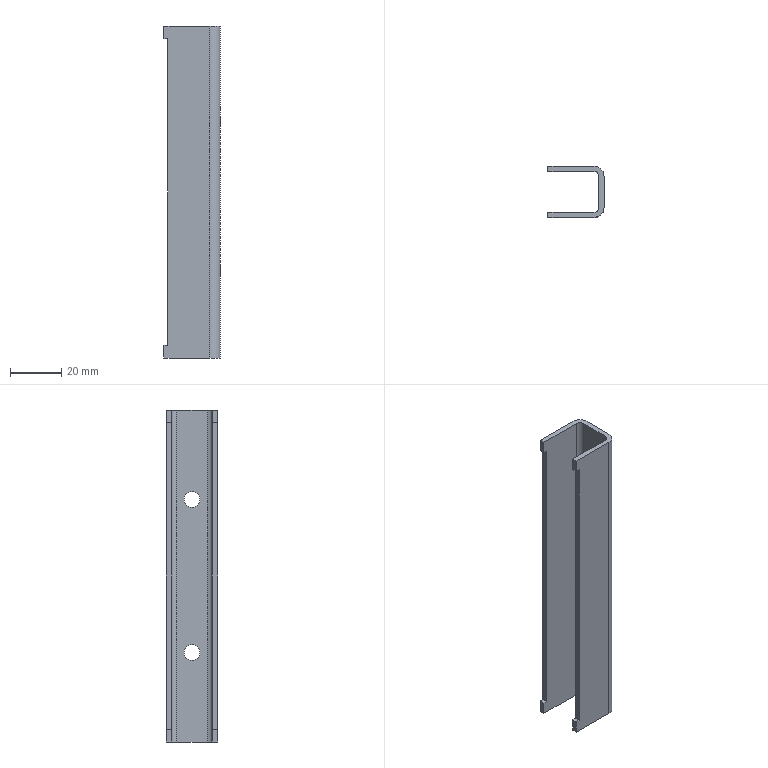Part | NX | features solid 2 | 1 solid | 26 faces | box 22 x 20 x 130 mm | volume 14090 mm3 | plane 18 | cylinder 8 | commonest cylinder face diameters 6.2 x4 4 x2 8 x2
STEP:
#1=CARTESIAN_POINT('',(-1108.,470.,587.));
#2=VERTEX_POINT('',#1);
#3=CARTESIAN_POINT('',(-1106.5,470.,587.));
#4=VERTEX_POINT('',#3);
#5=CARTESIAN_POINT('',(-1087.722,470.,587.));
#6=DIRECTION('',(1.,0.,0.));
#7=VECTOR('',#6,1000.);
#8=LINE('',#5,#7);
#9=EDGE_CURVE('',#2,#4,#8,.T.);
#10=ORIENTED_EDGE('',*,*,#9,.F.);
#11=CARTESIAN_POINT('',(-1108.,468.,587.));
#12=VERTEX_POINT('',#11);
#13=CARTESIAN_POINT('',(-1108.,468.,587.));
#14=DIRECTION('',(0.,-1.,0.));
#15=VECTOR('',#14,1000.);
#16=LINE('',#13,#15);
#17=EDGE_CURVE('',#2,#12,#16,.T.);
#18=ORIENTED_EDGE('',*,*,#17,.T.);
#19=CARTESIAN_POINT('',(-1106.5,468.,587.));
#20=VERTEX_POINT('',#19);
#21=CARTESIAN_POINT('',(-1087.722,468.,587.));
#22=DIRECTION('',(1.,0.,0.));
#23=VECTOR('',#22,1000.);
#24=LINE('',#21,#23);
#25=EDGE_CURVE('',#12,#20,#24,.T.);
#26=ORIENTED_EDGE('',*,*,#25,.T.);
#27=CARTESIAN_POINT('',(-1106.5,468.,587.));
#28=DIRECTION('',(0.,-1.,0.));
#29=VECTOR('',#28,1000.);
#30=LINE('',#27,#29);
#31=EDGE_CURVE('',#4,#20,#30,.T.);
#32=ORIENTED_EDGE('',*,*,#31,.F.);
#33=EDGE_LOOP('',(#10,#18,#26,#32));
#34=FACE_BOUND('',#33,.T.);
#35=CARTESIAN_POINT('',(-1087.722,468.,587.));
#36=DIRECTION('',(0.,0.,-1.));
#37=DIRECTION('',(-1.,0.,0.));
#38=AXIS2_PLACEMENT_3D('',#35,#36,#37);
#39=PLANE('',#38);
#40=ADVANCED_FACE('',(#34),#39,.F.);
#41=CARTESIAN_POINT('',(-1106.5,470.,707.));
#42=VERTEX_POINT('',#41);
#43=CARTESIAN_POINT('',(-1106.5,468.,707.));
#44=VERTEX_POINT('',#43);
#45=CARTESIAN_POINT('',(-1106.5,468.,707.));
#46=DIRECTION('',(0.,-1.,0.));
#47=VECTOR('',#46,1000.);
#48=LINE('',#45,#47);
#49=EDGE_CURVE('',#42,#44,#48,.T.);
#50=ORIENTED_EDGE('',*,*,#49,.T.);
#51=CARTESIAN_POINT('',(-1108.,468.,707.));
#52=VERTEX_POINT('',#51);
#53=CARTESIAN_POINT('',(-1087.722,468.,707.));
#54=DIRECTION('',(-1.,0.,0.));
#55=VECTOR('',#54,1000.);
#56=LINE('',#53,#55);
#57=EDGE_CURVE('',#44,#52,#56,.T.);
#58=ORIENTED_EDGE('',*,*,#57,.T.);
#59=CARTESIAN_POINT('',(-1108.,470.,707.));
#60=VERTEX_POINT('',#59);
#61=CARTESIAN_POINT('',(-1108.,468.,707.));
#62=DIRECTION('',(0.,-1.,0.));
#63=VECTOR('',#62,1000.);
#64=LINE('',#61,#63);
#65=EDGE_CURVE('',#60,#52,#64,.T.);
#66=ORIENTED_EDGE('',*,*,#65,.F.);
#67=CARTESIAN_POINT('',(-1087.722,470.,707.));
#68=DIRECTION('',(-1.,0.,0.));
#69=VECTOR('',#68,1000.);
#70=LINE('',#67,#69);
#71=EDGE_CURVE('',#42,#60,#70,.T.);
#72=ORIENTED_EDGE('',*,*,#71,.F.);
#73=EDGE_LOOP('',(#50,#58,#66,#72));
#74=FACE_BOUND('',#73,.T.);
#75=CARTESIAN_POINT('',(-1087.722,468.,707.));
#76=DIRECTION('',(0.,0.,1.));
#77=DIRECTION('',(1.,0.,0.));
#78=AXIS2_PLACEMENT_3D('',#75,#76,#77);
#79=PLANE('',#78);
#80=ADVANCED_FACE('',(#74),#79,.F.);
#81=ORIENTED_EDGE('',*,*,#31,.T.);
#82=CARTESIAN_POINT('',(-1106.5,468.,582.));
#83=DIRECTION('',(0.,0.,1.));
#84=VECTOR('',#83,1000.);
#85=LINE('',#82,#84);
#86=EDGE_CURVE('',#20,#44,#85,.T.);
#87=ORIENTED_EDGE('',*,*,#86,.T.);
#88=ORIENTED_EDGE('',*,*,#49,.F.);
#89=CARTESIAN_POINT('',(-1106.5,470.,582.));
#90=DIRECTION('',(0.,0.,1.));
#91=VECTOR('',#90,1000.);
#92=LINE('',#89,#91);
#93=EDGE_CURVE('',#4,#42,#92,.T.);
#94=ORIENTED_EDGE('',*,*,#93,.F.);
#95=EDGE_LOOP('',(#81,#87,#88,#94));
#96=FACE_BOUND('',#95,.T.);
#97=CARTESIAN_POINT('',(-1106.5,468.,582.));
#98=DIRECTION('',(1.,0.,0.));
#99=DIRECTION('',(0.,0.,1.));
#100=AXIS2_PLACEMENT_3D('',#97,#98,#99);
#101=PLANE('',#100);
#102=ADVANCED_FACE('',(#96),#101,.F.);
#103=CARTESIAN_POINT('',(-1106.5,486.,587.));
#104=VERTEX_POINT('',#103);
#105=CARTESIAN_POINT('',(-1108.,486.,587.));
#106=VERTEX_POINT('',#105);
#107=CARTESIAN_POINT('',(-1087.722,486.,587.));
#108=DIRECTION('',(-1.,0.,0.));
#109=VECTOR('',#108,1000.);
#110=LINE('',#107,#109);
#111=EDGE_CURVE('',#104,#106,#110,.T.);
#112=ORIENTED_EDGE('',*,*,#111,.F.);
#113=CARTESIAN_POINT('',(-1106.5,488.,587.));
#114=VERTEX_POINT('',#113);
#115=CARTESIAN_POINT('',(-1106.5,488.,587.));
#116=DIRECTION('',(0.,1.,0.));
#117=VECTOR('',#116,1000.);
#118=LINE('',#115,#117);
#119=EDGE_CURVE('',#104,#114,#118,.T.);
#120=ORIENTED_EDGE('',*,*,#119,.T.);
#121=CARTESIAN_POINT('',(-1108.,488.,587.));
#122=VERTEX_POINT('',#121);
#123=CARTESIAN_POINT('',(-1087.722,488.,587.));
#124=DIRECTION('',(-1.,0.,0.));
#125=VECTOR('',#124,1000.);
#126=LINE('',#123,#125);
#127=EDGE_CURVE('',#114,#122,#126,.T.);
#128=ORIENTED_EDGE('',*,*,#127,.T.);
#129=CARTESIAN_POINT('',(-1108.,488.,587.));
#130=DIRECTION('',(0.,1.,0.));
#131=VECTOR('',#130,1000.);
#132=LINE('',#129,#131);
#133=EDGE_CURVE('',#106,#122,#132,.T.);
#134=ORIENTED_EDGE('',*,*,#133,.F.);
#135=EDGE_LOOP('',(#112,#120,#128,#134));
#136=FACE_BOUND('',#135,.T.);
#137=CARTESIAN_POINT('',(-1087.722,488.,587.));
#138=DIRECTION('',(0.,0.,-1.));
#139=DIRECTION('',(-1.,0.,0.));
#140=AXIS2_PLACEMENT_3D('',#137,#138,#139);
#141=PLANE('',#140);
#142=ADVANCED_FACE('',(#136),#141,.F.);
#143=CARTESIAN_POINT('',(-1106.5,486.,707.));
#144=VERTEX_POINT('',#143);
#145=CARTESIAN_POINT('',(-1106.5,488.,707.));
#146=VERTEX_POINT('',#145);
#147=CARTESIAN_POINT('',(-1106.5,488.,707.));
#148=DIRECTION('',(0.,1.,0.));
#149=VECTOR('',#148,1000.);
#150=LINE('',#147,#149);
#151=EDGE_CURVE('',#144,#146,#150,.T.);
#152=ORIENTED_EDGE('',*,*,#151,.T.);
#153=CARTESIAN_POINT('',(-1106.5,488.,712.));
#154=DIRECTION('',(0.,0.,-1.));
#155=VECTOR('',#154,1000.);
#156=LINE('',#153,#155);
#157=EDGE_CURVE('',#146,#114,#156,.T.);
#158=ORIENTED_EDGE('',*,*,#157,.T.);
#159=ORIENTED_EDGE('',*,*,#119,.F.);
#160=CARTESIAN_POINT('',(-1106.5,486.,712.));
#161=DIRECTION('',(0.,0.,-1.));
#162=VECTOR('',#161,1000.);
#163=LINE('',#160,#162);
#164=EDGE_CURVE('',#144,#104,#163,.T.);
#165=ORIENTED_EDGE('',*,*,#164,.F.);
#166=EDGE_LOOP('',(#152,#158,#159,#165));
#167=FACE_BOUND('',#166,.T.);
#168=CARTESIAN_POINT('',(-1106.5,488.,712.));
#169=DIRECTION('',(1.,0.,0.));
#170=DIRECTION('',(0.,0.,1.));
#171=AXIS2_PLACEMENT_3D('',#168,#169,#170);
#172=PLANE('',#171);
#173=ADVANCED_FACE('',(#167),#172,.F.);
#174=CARTESIAN_POINT('',(-1108.,486.,707.));
#175=VERTEX_POINT('',#174);
#176=CARTESIAN_POINT('',(-1108.,488.,707.));
#177=VERTEX_POINT('',#176);
#178=CARTESIAN_POINT('',(-1108.,488.,707.));
#179=DIRECTION('',(0.,1.,0.));
#180=VECTOR('',#179,1000.);
#181=LINE('',#178,#180);
#182=EDGE_CURVE('',#175,#177,#181,.T.);
#183=ORIENTED_EDGE('',*,*,#182,.T.);
#184=CARTESIAN_POINT('',(-1087.722,488.,707.));
#185=DIRECTION('',(1.,0.,0.));
#186=VECTOR('',#185,1000.);
#187=LINE('',#184,#186);
#188=EDGE_CURVE('',#177,#146,#187,.T.);
#189=ORIENTED_EDGE('',*,*,#188,.T.);
#190=ORIENTED_EDGE('',*,*,#151,.F.);
#191=CARTESIAN_POINT('',(-1087.722,486.,707.));
#192=DIRECTION('',(1.,0.,0.));
#193=VECTOR('',#192,1000.);
#194=LINE('',#191,#193);
#195=EDGE_CURVE('',#175,#144,#194,.T.);
#196=ORIENTED_EDGE('',*,*,#195,.F.);
#197=EDGE_LOOP('',(#183,#189,#190,#196));
#198=FACE_BOUND('',#197,.T.);
#199=CARTESIAN_POINT('',(-1087.722,488.,707.));
#200=DIRECTION('',(0.,0.,1.));
#201=DIRECTION('',(1.,0.,0.));
#202=AXIS2_PLACEMENT_3D('',#199,#200,#201);
#203=PLANE('',#202);
#204=ADVANCED_FACE('',(#198),#203,.F.);
#205=CARTESIAN_POINT('',(-1088.,484.,582.));
#206=VERTEX_POINT('',#205);
#207=CARTESIAN_POINT('',(-1088.,484.,712.));
#208=VERTEX_POINT('',#207);
#209=CARTESIAN_POINT('',(-1088.,484.,582.));
#210=DIRECTION('',(0.,0.,1.));
#211=VECTOR('',#210,1000.);
#212=LINE('',#209,#211);
#213=EDGE_CURVE('',#206,#208,#212,.T.);
#214=ORIENTED_EDGE('',*,*,#213,.T.);
#215=CARTESIAN_POINT('',(-1090.,486.,712.));
#216=VERTEX_POINT('',#215);
#217=CARTESIAN_POINT('',(-1090.,484.,712.));
#218=DIRECTION('',(0.,0.,1.));
#219=DIRECTION('',(0.,-1.,0.));
#220=AXIS2_PLACEMENT_3D('',#217,#218,#219);
#221=CIRCLE('',#220,2.);
#222=EDGE_CURVE('',#208,#216,#221,.T.);
#223=ORIENTED_EDGE('',*,*,#222,.T.);
#224=CARTESIAN_POINT('',(-1090.,486.,582.));
#225=VERTEX_POINT('',#224);
#226=CARTESIAN_POINT('',(-1090.,486.,712.));
#227=DIRECTION('',(0.,0.,-1.));
#228=VECTOR('',#227,1000.);
#229=LINE('',#226,#228);
#230=EDGE_CURVE('',#216,#225,#229,.T.);
#231=ORIENTED_EDGE('',*,*,#230,.T.);
#232=CARTESIAN_POINT('',(-1090.,484.,582.));
#233=DIRECTION('',(0.,0.,-1.));
#234=DIRECTION('',(0.,-1.,0.));
#235=AXIS2_PLACEMENT_3D('',#232,#233,#234);
#236=CIRCLE('',#235,2.);
#237=EDGE_CURVE('',#225,#206,#236,.T.);
#238=ORIENTED_EDGE('',*,*,#237,.T.);
#239=EDGE_LOOP('',(#214,#223,#231,#238));
#240=FACE_BOUND('',#239,.T.);
#241=CARTESIAN_POINT('',(-1090.,484.,582.));
#242=DIRECTION('',(0.,0.,1.));
#243=DIRECTION('',(-1.,0.,0.));
#244=AXIS2_PLACEMENT_3D('',#241,#242,#243);
#245=CYLINDRICAL_SURFACE('',#244,2.);
#246=ADVANCED_FACE('',(#240),#245,.F.);
#247=CARTESIAN_POINT('',(-1086.,484.,582.));
#248=VERTEX_POINT('',#247);
#249=CARTESIAN_POINT('',(-1086.,484.,712.));
#250=VERTEX_POINT('',#249);
#251=CARTESIAN_POINT('',(-1086.,484.,582.));
#252=DIRECTION('',(0.,0.,1.));
#253=VECTOR('',#252,1000.);
#254=LINE('',#251,#253);
#255=EDGE_CURVE('',#248,#250,#254,.T.);
#256=ORIENTED_EDGE('',*,*,#255,.F.);
#257=CARTESIAN_POINT('',(-1090.,488.,582.));
#258=VERTEX_POINT('',#257);
#259=CARTESIAN_POINT('',(-1090.,484.,582.));
#260=DIRECTION('',(0.,0.,-1.));
#261=DIRECTION('',(-1.,0.,0.));
#262=AXIS2_PLACEMENT_3D('',#259,#260,#261);
#263=CIRCLE('',#262,4.);
#264=EDGE_CURVE('',#258,#248,#263,.T.);
#265=ORIENTED_EDGE('',*,*,#264,.F.);
#266=CARTESIAN_POINT('',(-1090.,488.,712.));
#267=VERTEX_POINT('',#266);
#268=CARTESIAN_POINT('',(-1090.,488.,712.));
#269=DIRECTION('',(0.,0.,-1.));
#270=VECTOR('',#269,1000.);
#271=LINE('',#268,#270);
#272=EDGE_CURVE('',#267,#258,#271,.T.);
#273=ORIENTED_EDGE('',*,*,#272,.F.);
#274=CARTESIAN_POINT('',(-1090.,484.,712.));
#275=DIRECTION('',(0.,0.,1.));
#276=DIRECTION('',(-1.,0.,0.));
#277=AXIS2_PLACEMENT_3D('',#274,#275,#276);
#278=CIRCLE('',#277,4.);
#279=EDGE_CURVE('',#250,#267,#278,.T.);
#280=ORIENTED_EDGE('',*,*,#279,.F.);
#281=EDGE_LOOP('',(#256,#265,#273,#280));
#282=FACE_BOUND('',#281,.T.);
#283=CARTESIAN_POINT('',(-1090.,484.,582.));
#284=DIRECTION('',(0.,0.,1.));
#285=DIRECTION('',(-1.,0.,0.));
#286=AXIS2_PLACEMENT_3D('',#283,#284,#285);
#287=CYLINDRICAL_SURFACE('',#286,4.);
#288=ADVANCED_FACE('',(#282),#287,.T.);
#289=CARTESIAN_POINT('',(-1108.,486.,582.));
#290=VERTEX_POINT('',#289);
#291=CARTESIAN_POINT('',(-1108.,486.,582.));
#292=DIRECTION('',(0.,0.,1.));
#293=VECTOR('',#292,1000.);
#294=LINE('',#291,#293);
#295=EDGE_CURVE('',#290,#106,#294,.T.);
#296=ORIENTED_EDGE('',*,*,#295,.T.);
#297=ORIENTED_EDGE('',*,*,#133,.T.);
#298=CARTESIAN_POINT('',(-1108.,488.,582.));
#299=VERTEX_POINT('',#298);
#300=CARTESIAN_POINT('',(-1108.,488.,582.));
#301=DIRECTION('',(0.,0.,1.));
#302=VECTOR('',#301,1000.);
#303=LINE('',#300,#302);
#304=EDGE_CURVE('',#299,#122,#303,.T.);
#305=ORIENTED_EDGE('',*,*,#304,.F.);
#306=CARTESIAN_POINT('',(-1108.,488.,582.));
#307=DIRECTION('',(0.,-1.,0.));
#308=VECTOR('',#307,1000.);
#309=LINE('',#306,#308);
#310=EDGE_CURVE('',#299,#290,#309,.T.);
#311=ORIENTED_EDGE('',*,*,#310,.T.);
#312=EDGE_LOOP('',(#296,#297,#305,#311));
#313=FACE_BOUND('',#312,.T.);
#314=CARTESIAN_POINT('',(-1108.,488.,582.));
#315=DIRECTION('',(1.,0.,0.));
#316=DIRECTION('',(0.,0.,1.));
#317=AXIS2_PLACEMENT_3D('',#314,#315,#316);
#318=PLANE('',#317);
#319=ADVANCED_FACE('',(#313),#318,.F.);
#320=CARTESIAN_POINT('',(-1108.,486.,712.));
#321=VERTEX_POINT('',#320);
#322=CARTESIAN_POINT('',(-1108.,486.,582.));
#323=DIRECTION('',(0.,0.,1.));
#324=VECTOR('',#323,1000.);
#325=LINE('',#322,#324);
#326=EDGE_CURVE('',#175,#321,#325,.T.);
#327=ORIENTED_EDGE('',*,*,#326,.F.);
#328=ORIENTED_EDGE('',*,*,#195,.T.);
#329=ORIENTED_EDGE('',*,*,#164,.T.);
#330=ORIENTED_EDGE('',*,*,#111,.T.);
#331=ORIENTED_EDGE('',*,*,#295,.F.);
#332=CARTESIAN_POINT('',(-1087.722,486.,582.));
#333=DIRECTION('',(-1.,0.,0.));
#334=VECTOR('',#333,1000.);
#335=LINE('',#332,#334);
#336=EDGE_CURVE('',#225,#290,#335,.T.);
#337=ORIENTED_EDGE('',*,*,#336,.F.);
#338=ORIENTED_EDGE('',*,*,#230,.F.);
#339=CARTESIAN_POINT('',(-1087.722,486.,712.));
#340=DIRECTION('',(1.,0.,0.));
#341=VECTOR('',#340,1000.);
#342=LINE('',#339,#341);
#343=EDGE_CURVE('',#321,#216,#342,.T.);
#344=ORIENTED_EDGE('',*,*,#343,.F.);
#345=EDGE_LOOP('',(#327,#328,#329,#330,#331,#337,#338,#344));
#346=FACE_BOUND('',#345,.T.);
#347=CARTESIAN_POINT('',(-1087.722,486.,712.));
#348=DIRECTION('',(0.,1.,0.));
#349=DIRECTION('',(0.,0.,-1.));
#350=AXIS2_PLACEMENT_3D('',#347,#348,#349);
#351=PLANE('',#350);
#352=ADVANCED_FACE('',(#346),#351,.F.);
#353=ORIENTED_EDGE('',*,*,#188,.F.);
#354=CARTESIAN_POINT('',(-1108.,488.,712.));
#355=VERTEX_POINT('',#354);
#356=CARTESIAN_POINT('',(-1108.,488.,582.));
#357=DIRECTION('',(0.,0.,1.));
#358=VECTOR('',#357,1000.);
#359=LINE('',#356,#358);
#360=EDGE_CURVE('',#177,#355,#359,.T.);
#361=ORIENTED_EDGE('',*,*,#360,.T.);
#362=CARTESIAN_POINT('',(-1087.722,488.,712.));
#363=DIRECTION('',(1.,0.,0.));
#364=VECTOR('',#363,1000.);
#365=LINE('',#362,#364);
#366=EDGE_CURVE('',#355,#267,#365,.T.);
#367=ORIENTED_EDGE('',*,*,#366,.T.);
#368=ORIENTED_EDGE('',*,*,#272,.T.);
#369=CARTESIAN_POINT('',(-1087.722,488.,582.));
#370=DIRECTION('',(-1.,0.,0.));
#371=VECTOR('',#370,1000.);
#372=LINE('',#369,#371);
#373=EDGE_CURVE('',#258,#299,#372,.T.);
#374=ORIENTED_EDGE('',*,*,#373,.T.);
#375=ORIENTED_EDGE('',*,*,#304,.T.);
#376=ORIENTED_EDGE('',*,*,#127,.F.);
#377=ORIENTED_EDGE('',*,*,#157,.F.);
#378=EDGE_LOOP('',(#353,#361,#367,#368,#374,#375,#376,#377));
#379=FACE_BOUND('',#378,.T.);
#380=CARTESIAN_POINT('',(-1087.722,488.,712.));
#381=DIRECTION('',(0.,1.,0.));
#382=DIRECTION('',(0.,0.,-1.));
#383=AXIS2_PLACEMENT_3D('',#380,#381,#382);
#384=PLANE('',#383);
#385=ADVANCED_FACE('',(#379),#384,.T.);
#386=CARTESIAN_POINT('',(-1088.,472.,712.));
#387=VERTEX_POINT('',#386);
#388=CARTESIAN_POINT('',(-1088.,472.,582.));
#389=VERTEX_POINT('',#388);
#390=CARTESIAN_POINT('',(-1088.,472.,712.));
#391=DIRECTION('',(0.,0.,-1.));
#392=VECTOR('',#391,1000.);
#393=LINE('',#390,#392);
#394=EDGE_CURVE('',#387,#389,#393,.T.);
#395=ORIENTED_EDGE('',*,*,#394,.T.);
#396=CARTESIAN_POINT('',(-1090.,470.,582.));
#397=VERTEX_POINT('',#396);
#398=CARTESIAN_POINT('',(-1090.,472.,582.));
#399=DIRECTION('',(0.,0.,-1.));
#400=DIRECTION('',(0.,1.,0.));
#401=AXIS2_PLACEMENT_3D('',#398,#399,#400);
#402=CIRCLE('',#401,2.);
#403=EDGE_CURVE('',#389,#397,#402,.T.);
#404=ORIENTED_EDGE('',*,*,#403,.T.);
#405=CARTESIAN_POINT('',(-1090.,470.,712.));
#406=VERTEX_POINT('',#405);
#407=CARTESIAN_POINT('',(-1090.,470.,582.));
#408=DIRECTION('',(0.,0.,1.));
#409=VECTOR('',#408,1000.);
#410=LINE('',#407,#409);
#411=EDGE_CURVE('',#397,#406,#410,.T.);
#412=ORIENTED_EDGE('',*,*,#411,.T.);
#413=CARTESIAN_POINT('',(-1090.,472.,712.));
#414=DIRECTION('',(0.,0.,1.));
#415=DIRECTION('',(0.,1.,0.));
#416=AXIS2_PLACEMENT_3D('',#413,#414,#415);
#417=CIRCLE('',#416,2.);
#418=EDGE_CURVE('',#406,#387,#417,.T.);
#419=ORIENTED_EDGE('',*,*,#418,.T.);
#420=EDGE_LOOP('',(#395,#404,#412,#419));
#421=FACE_BOUND('',#420,.T.);
#422=CARTESIAN_POINT('',(-1090.,472.,712.));
#423=DIRECTION('',(0.,0.,-1.));
#424=DIRECTION('',(-1.,0.,0.));
#425=AXIS2_PLACEMENT_3D('',#422,#423,#424);
#426=CYLINDRICAL_SURFACE('',#425,2.);
#427=ADVANCED_FACE('',(#421),#426,.F.);
#428=CARTESIAN_POINT('',(-1086.,472.,712.));
#429=VERTEX_POINT('',#428);
#430=CARTESIAN_POINT('',(-1086.,472.,582.));
#431=VERTEX_POINT('',#430);
#432=CARTESIAN_POINT('',(-1086.,472.,712.));
#433=DIRECTION('',(0.,0.,-1.));
#434=VECTOR('',#433,1000.);
#435=LINE('',#432,#434);
#436=EDGE_CURVE('',#429,#431,#435,.T.);
#437=ORIENTED_EDGE('',*,*,#436,.F.);
#438=CARTESIAN_POINT('',(-1090.,468.,712.));
#439=VERTEX_POINT('',#438);
#440=CARTESIAN_POINT('',(-1090.,472.,712.));
#441=DIRECTION('',(0.,0.,1.));
#442=DIRECTION('',(-1.,0.,0.));
#443=AXIS2_PLACEMENT_3D('',#440,#441,#442);
#444=CIRCLE('',#443,4.);
#445=EDGE_CURVE('',#439,#429,#444,.T.);
#446=ORIENTED_EDGE('',*,*,#445,.F.);
#447=CARTESIAN_POINT('',(-1090.,468.,582.));
#448=VERTEX_POINT('',#447);
#449=CARTESIAN_POINT('',(-1090.,468.,582.));
#450=DIRECTION('',(0.,0.,1.));
#451=VECTOR('',#450,1000.);
#452=LINE('',#449,#451);
#453=EDGE_CURVE('',#448,#439,#452,.T.);
#454=ORIENTED_EDGE('',*,*,#453,.F.);
#455=CARTESIAN_POINT('',(-1090.,472.,582.));
#456=DIRECTION('',(0.,0.,-1.));
#457=DIRECTION('',(-1.,0.,0.));
#458=AXIS2_PLACEMENT_3D('',#455,#456,#457);
#459=CIRCLE('',#458,4.);
#460=EDGE_CURVE('',#431,#448,#459,.T.);
#461=ORIENTED_EDGE('',*,*,#460,.F.);
#462=EDGE_LOOP('',(#437,#446,#454,#461));
#463=FACE_BOUND('',#462,.T.);
#464=CARTESIAN_POINT('',(-1090.,472.,712.));
#465=DIRECTION('',(0.,0.,-1.));
#466=DIRECTION('',(-1.,0.,0.));
#467=AXIS2_PLACEMENT_3D('',#464,#465,#466);
#468=CYLINDRICAL_SURFACE('',#467,4.);
#469=ADVANCED_FACE('',(#463),#468,.T.);
#470=CARTESIAN_POINT('',(-1108.,468.,582.));
#471=VERTEX_POINT('',#470);
#472=CARTESIAN_POINT('',(-1108.,468.,712.));
#473=DIRECTION('',(0.,0.,-1.));
#474=VECTOR('',#473,1000.);
#475=LINE('',#472,#474);
#476=EDGE_CURVE('',#12,#471,#475,.T.);
#477=ORIENTED_EDGE('',*,*,#476,.F.);
#478=ORIENTED_EDGE('',*,*,#17,.F.);
#479=CARTESIAN_POINT('',(-1108.,470.,582.));
#480=VERTEX_POINT('',#479);
#481=CARTESIAN_POINT('',(-1108.,470.,712.));
#482=DIRECTION('',(0.,0.,-1.));
#483=VECTOR('',#482,1000.);
#484=LINE('',#481,#483);
#485=EDGE_CURVE('',#2,#480,#484,.T.);
#486=ORIENTED_EDGE('',*,*,#485,.T.);
#487=CARTESIAN_POINT('',(-1108.,468.,582.));
#488=DIRECTION('',(0.,1.,0.));
#489=VECTOR('',#488,1000.);
#490=LINE('',#487,#489);
#491=EDGE_CURVE('',#471,#480,#490,.T.);
#492=ORIENTED_EDGE('',*,*,#491,.F.);
#493=EDGE_LOOP('',(#477,#478,#486,#492));
#494=FACE_BOUND('',#493,.T.);
#495=CARTESIAN_POINT('',(-1108.,468.,712.));
#496=DIRECTION('',(1.,0.,0.));
#497=DIRECTION('',(0.,0.,1.));
#498=AXIS2_PLACEMENT_3D('',#495,#496,#497);
#499=PLANE('',#498);
#500=ADVANCED_FACE('',(#494),#499,.F.);
#501=ORIENTED_EDGE('',*,*,#93,.T.);
#502=ORIENTED_EDGE('',*,*,#71,.T.);
#503=CARTESIAN_POINT('',(-1108.,470.,712.));
#504=VERTEX_POINT('',#503);
#505=CARTESIAN_POINT('',(-1108.,470.,712.));
#506=DIRECTION('',(0.,0.,-1.));
#507=VECTOR('',#506,1000.);
#508=LINE('',#505,#507);
#509=EDGE_CURVE('',#504,#60,#508,.T.);
#510=ORIENTED_EDGE('',*,*,#509,.F.);
#511=CARTESIAN_POINT('',(-1087.722,470.,712.));
#512=DIRECTION('',(-1.,0.,0.));
#513=VECTOR('',#512,1000.);
#514=LINE('',#511,#513);
#515=EDGE_CURVE('',#406,#504,#514,.T.);
#516=ORIENTED_EDGE('',*,*,#515,.F.);
#517=ORIENTED_EDGE('',*,*,#411,.F.);
#518=CARTESIAN_POINT('',(-1087.722,470.,582.));
#519=DIRECTION('',(1.,0.,0.));
#520=VECTOR('',#519,1000.);
#521=LINE('',#518,#520);
#522=EDGE_CURVE('',#480,#397,#521,.T.);
#523=ORIENTED_EDGE('',*,*,#522,.F.);
#524=ORIENTED_EDGE('',*,*,#485,.F.);
#525=ORIENTED_EDGE('',*,*,#9,.T.);
#526=EDGE_LOOP('',(#501,#502,#510,#516,#517,#523,#524,#525));
#527=FACE_BOUND('',#526,.T.);
#528=CARTESIAN_POINT('',(-1087.722,470.,582.));
#529=DIRECTION('',(0.,-1.,0.));
#530=DIRECTION('',(0.,0.,-1.));
#531=AXIS2_PLACEMENT_3D('',#528,#529,#530);
#532=PLANE('',#531);
#533=ADVANCED_FACE('',(#527),#532,.F.);
#534=ORIENTED_EDGE('',*,*,#57,.F.);
#535=ORIENTED_EDGE('',*,*,#86,.F.);
#536=ORIENTED_EDGE('',*,*,#25,.F.);
#537=ORIENTED_EDGE('',*,*,#476,.T.);
#538=CARTESIAN_POINT('',(-1087.722,468.,582.));
#539=DIRECTION('',(1.,0.,0.));
#540=VECTOR('',#539,1000.);
#541=LINE('',#538,#540);
#542=EDGE_CURVE('',#471,#448,#541,.T.);
#543=ORIENTED_EDGE('',*,*,#542,.T.);
#544=ORIENTED_EDGE('',*,*,#453,.T.);
#545=CARTESIAN_POINT('',(-1108.,468.,712.));
#546=VERTEX_POINT('',#545);
#547=CARTESIAN_POINT('',(-1087.722,468.,712.));
#548=DIRECTION('',(-1.,0.,0.));
#549=VECTOR('',#548,1000.);
#550=LINE('',#547,#549);
#551=EDGE_CURVE('',#439,#546,#550,.T.);
#552=ORIENTED_EDGE('',*,*,#551,.T.);
#553=CARTESIAN_POINT('',(-1108.,468.,712.));
#554=DIRECTION('',(0.,0.,-1.));
#555=VECTOR('',#554,1000.);
#556=LINE('',#553,#555);
#557=EDGE_CURVE('',#546,#52,#556,.T.);
#558=ORIENTED_EDGE('',*,*,#557,.T.);
#559=EDGE_LOOP('',(#534,#535,#536,#537,#543,#544,#552,#558));
#560=FACE_BOUND('',#559,.T.);
#561=CARTESIAN_POINT('',(-1087.722,468.,582.));
#562=DIRECTION('',(0.,-1.,0.));
#563=DIRECTION('',(0.,0.,-1.));
#564=AXIS2_PLACEMENT_3D('',#561,#562,#563);
#565=PLANE('',#564);
#566=ADVANCED_FACE('',(#560),#565,.T.);
#567=CARTESIAN_POINT('',(-1088.,478.,680.1));
#568=VERTEX_POINT('',#567);
#569=CARTESIAN_POINT('',(-1086.,478.,680.1));
#570=VERTEX_POINT('',#569);
#571=CARTESIAN_POINT('',(-956.455,478.,680.1));
#572=DIRECTION('',(-1.,0.,0.));
#573=VECTOR('',#572,1000.);
#574=LINE('',#571,#573);
#575=EDGE_CURVE('',#568,#570,#574,.F.);
#576=ORIENTED_EDGE('',*,*,#575,.T.);
#577=CARTESIAN_POINT('',(-1086.,478.,673.9));
#578=VERTEX_POINT('',#577);
#579=CARTESIAN_POINT('',(-1086.,478.,677.));
#580=DIRECTION('',(-1.,0.,0.));
#581=DIRECTION('',(0.,0.,-1.));
#582=AXIS2_PLACEMENT_3D('',#579,#580,#581);
#583=CIRCLE('',#582,3.1);
#584=EDGE_CURVE('',#578,#570,#583,.T.);
#585=ORIENTED_EDGE('',*,*,#584,.F.);
#586=CARTESIAN_POINT('',(-1088.,478.,673.9));
#587=VERTEX_POINT('',#586);
#588=CARTESIAN_POINT('',(-956.455,478.,673.9));
#589=DIRECTION('',(-1.,0.,0.));
#590=VECTOR('',#589,1000.);
#591=LINE('',#588,#590);
#592=EDGE_CURVE('',#578,#587,#591,.T.);
#593=ORIENTED_EDGE('',*,*,#592,.T.);
#594=CARTESIAN_POINT('',(-1088.,478.,677.));
#595=DIRECTION('',(-1.,0.,0.));
#596=DIRECTION('',(0.,0.,-1.));
#597=AXIS2_PLACEMENT_3D('',#594,#595,#596);
#598=CIRCLE('',#597,3.1);
#599=EDGE_CURVE('',#587,#568,#598,.T.);
#600=ORIENTED_EDGE('',*,*,#599,.T.);
#601=EDGE_LOOP('',(#576,#585,#593,#600));
#602=FACE_BOUND('',#601,.T.);
#603=CARTESIAN_POINT('',(-956.455,478.,677.));
#604=DIRECTION('',(-1.,0.,0.));
#605=DIRECTION('',(0.,0.,-1.));
#606=AXIS2_PLACEMENT_3D('',#603,#604,#605);
#607=CYLINDRICAL_SURFACE('',#606,3.1);
#608=ADVANCED_FACE('',(#602),#607,.F.);
#609=CARTESIAN_POINT('',(-1086.,478.,620.1));
#610=VERTEX_POINT('',#609);
#611=CARTESIAN_POINT('',(-1088.,478.,620.1));
#612=VERTEX_POINT('',#611);
#613=CARTESIAN_POINT('',(-956.455,478.,620.1));
#614=DIRECTION('',(-1.,0.,0.));
#615=VECTOR('',#614,1000.);
#616=LINE('',#613,#615);
#617=EDGE_CURVE('',#610,#612,#616,.T.);
#618=ORIENTED_EDGE('',*,*,#617,.F.);
#619=CARTESIAN_POINT('',(-1086.,478.,613.9));
#620=VERTEX_POINT('',#619);
#621=CARTESIAN_POINT('',(-1086.,478.,617.));
#622=DIRECTION('',(-1.,0.,0.));
#623=DIRECTION('',(0.,0.,-1.));
#624=AXIS2_PLACEMENT_3D('',#621,#622,#623);
#625=CIRCLE('',#624,3.1);
#626=EDGE_CURVE('',#620,#610,#625,.T.);
#627=ORIENTED_EDGE('',*,*,#626,.F.);
#628=CARTESIAN_POINT('',(-1088.,478.,613.9));
#629=VERTEX_POINT('',#628);
#630=CARTESIAN_POINT('',(-956.455,478.,613.9));
#631=DIRECTION('',(-1.,0.,0.));
#632=VECTOR('',#631,1000.);
#633=LINE('',#630,#632);
#634=EDGE_CURVE('',#629,#620,#633,.F.);
#635=ORIENTED_EDGE('',*,*,#634,.F.);
#636=CARTESIAN_POINT('',(-1088.,478.,617.));
#637=DIRECTION('',(-1.,0.,0.));
#638=DIRECTION('',(0.,0.,-1.));
#639=AXIS2_PLACEMENT_3D('',#636,#637,#638);
#640=CIRCLE('',#639,3.1);
#641=EDGE_CURVE('',#629,#612,#640,.T.);
#642=ORIENTED_EDGE('',*,*,#641,.T.);
#643=EDGE_LOOP('',(#618,#627,#635,#642));
#644=FACE_BOUND('',#643,.T.);
#645=CARTESIAN_POINT('',(-956.455,478.,617.));
#646=DIRECTION('',(-1.,0.,0.));
#647=DIRECTION('',(0.,0.,-1.));
#648=AXIS2_PLACEMENT_3D('',#645,#646,#647);
#649=CYLINDRICAL_SURFACE('',#648,3.1);
#650=ADVANCED_FACE('',(#644),#649,.F.);
#651=ORIENTED_EDGE('',*,*,#641,.F.);
#652=CARTESIAN_POINT('',(-1088.,478.,617.));
#653=DIRECTION('',(-1.,0.,0.));
#654=DIRECTION('',(0.,0.,-1.));
#655=AXIS2_PLACEMENT_3D('',#652,#653,#654);
#656=CIRCLE('',#655,3.1);
#657=EDGE_CURVE('',#612,#629,#656,.T.);
#658=ORIENTED_EDGE('',*,*,#657,.F.);
#659=EDGE_LOOP('',(#651,#658));
#660=FACE_BOUND('',#659,.T.);
#661=ORIENTED_EDGE('',*,*,#599,.F.);
#662=CARTESIAN_POINT('',(-1088.,478.,677.));
#663=DIRECTION('',(-1.,0.,0.));
#664=DIRECTION('',(0.,0.,-1.));
#665=AXIS2_PLACEMENT_3D('',#662,#663,#664);
#666=CIRCLE('',#665,3.1);
#667=EDGE_CURVE('',#568,#587,#666,.T.);
#668=ORIENTED_EDGE('',*,*,#667,.F.);
#669=EDGE_LOOP('',(#661,#668));
#670=FACE_BOUND('',#669,.T.);
#671=ORIENTED_EDGE('',*,*,#213,.F.);
#672=CARTESIAN_POINT('',(-1088.,488.,582.));
#673=DIRECTION('',(0.,-1.,0.));
#674=VECTOR('',#673,1000.);
#675=LINE('',#672,#674);
#676=EDGE_CURVE('',#206,#389,#675,.T.);
#677=ORIENTED_EDGE('',*,*,#676,.T.);
#678=ORIENTED_EDGE('',*,*,#394,.F.);
#679=CARTESIAN_POINT('',(-1088.,468.,712.));
#680=DIRECTION('',(0.,1.,0.));
#681=VECTOR('',#680,1000.);
#682=LINE('',#679,#681);
#683=EDGE_CURVE('',#387,#208,#682,.T.);
#684=ORIENTED_EDGE('',*,*,#683,.T.);
#685=EDGE_LOOP('',(#671,#677,#678,#684));
#686=FACE_BOUND('',#685,.T.);
#687=CARTESIAN_POINT('',(-1088.,488.,582.));
#688=DIRECTION('',(-1.,0.,0.));
#689=DIRECTION('',(0.,0.,1.));
#690=AXIS2_PLACEMENT_3D('',#687,#688,#689);
#691=PLANE('',#690);
#692=ADVANCED_FACE('',(#660,#670,#686),#691,.T.);
#693=ORIENTED_EDGE('',*,*,#626,.T.);
#694=CARTESIAN_POINT('',(-1086.,478.,617.));
#695=DIRECTION('',(-1.,0.,0.));
#696=DIRECTION('',(0.,0.,-1.));
#697=AXIS2_PLACEMENT_3D('',#694,#695,#696);
#698=CIRCLE('',#697,3.1);
#699=EDGE_CURVE('',#610,#620,#698,.T.);
#700=ORIENTED_EDGE('',*,*,#699,.T.);
#701=EDGE_LOOP('',(#693,#700));
#702=FACE_BOUND('',#701,.T.);
#703=ORIENTED_EDGE('',*,*,#584,.T.);
#704=CARTESIAN_POINT('',(-1086.,478.,677.));
#705=DIRECTION('',(-1.,0.,0.));
#706=DIRECTION('',(0.,0.,-1.));
#707=AXIS2_PLACEMENT_3D('',#704,#705,#706);
#708=CIRCLE('',#707,3.1);
#709=EDGE_CURVE('',#570,#578,#708,.T.);
#710=ORIENTED_EDGE('',*,*,#709,.T.);
#711=EDGE_LOOP('',(#703,#710));
#712=FACE_BOUND('',#711,.T.);
#713=CARTESIAN_POINT('',(-1086.,488.,582.));
#714=DIRECTION('',(0.,-1.,0.));
#715=VECTOR('',#714,1000.);
#716=LINE('',#713,#715);
#717=EDGE_CURVE('',#248,#431,#716,.T.);
#718=ORIENTED_EDGE('',*,*,#717,.F.);
#719=ORIENTED_EDGE('',*,*,#255,.T.);
#720=CARTESIAN_POINT('',(-1086.,468.,712.));
#721=DIRECTION('',(0.,1.,0.));
#722=VECTOR('',#721,1000.);
#723=LINE('',#720,#722);
#724=EDGE_CURVE('',#429,#250,#723,.T.);
#725=ORIENTED_EDGE('',*,*,#724,.F.);
#726=ORIENTED_EDGE('',*,*,#436,.T.);
#727=EDGE_LOOP('',(#718,#719,#725,#726));
#728=FACE_BOUND('',#727,.T.);
#729=CARTESIAN_POINT('',(-1086.,488.,582.));
#730=DIRECTION('',(-1.,0.,0.));
#731=DIRECTION('',(0.,0.,1.));
#732=AXIS2_PLACEMENT_3D('',#729,#730,#731);
#733=PLANE('',#732);
#734=ADVANCED_FACE('',(#702,#712,#728),#733,.F.);
#735=ORIENTED_EDGE('',*,*,#724,.T.);
#736=ORIENTED_EDGE('',*,*,#279,.T.);
#737=ORIENTED_EDGE('',*,*,#366,.F.);
#738=CARTESIAN_POINT('',(-1108.,488.,712.));
#739=DIRECTION('',(0.,-1.,0.));
#740=VECTOR('',#739,1000.);
#741=LINE('',#738,#740);
#742=EDGE_CURVE('',#355,#321,#741,.T.);
#743=ORIENTED_EDGE('',*,*,#742,.T.);
#744=ORIENTED_EDGE('',*,*,#343,.T.);
#745=ORIENTED_EDGE('',*,*,#222,.F.);
#746=ORIENTED_EDGE('',*,*,#683,.F.);
#747=ORIENTED_EDGE('',*,*,#418,.F.);
#748=ORIENTED_EDGE('',*,*,#515,.T.);
#749=CARTESIAN_POINT('',(-1108.,468.,712.));
#750=DIRECTION('',(0.,1.,0.));
#751=VECTOR('',#750,1000.);
#752=LINE('',#749,#751);
#753=EDGE_CURVE('',#546,#504,#752,.T.);
#754=ORIENTED_EDGE('',*,*,#753,.F.);
#755=ORIENTED_EDGE('',*,*,#551,.F.);
#756=ORIENTED_EDGE('',*,*,#445,.T.);
#757=EDGE_LOOP('',(#735,#736,#737,#743,#744,#745,#746,#747,#748,#754,#755,#756));
#758=FACE_BOUND('',#757,.T.);
#759=CARTESIAN_POINT('',(-1088.,468.,712.));
#760=DIRECTION('',(0.,0.,-1.));
#761=DIRECTION('',(-1.,0.,0.));
#762=AXIS2_PLACEMENT_3D('',#759,#760,#761);
#763=PLANE('',#762);
#764=ADVANCED_FACE('',(#758),#763,.F.);
#765=ORIENTED_EDGE('',*,*,#676,.F.);
#766=ORIENTED_EDGE('',*,*,#237,.F.);
#767=ORIENTED_EDGE('',*,*,#336,.T.);
#768=ORIENTED_EDGE('',*,*,#310,.F.);
#769=ORIENTED_EDGE('',*,*,#373,.F.);
#770=ORIENTED_EDGE('',*,*,#264,.T.);
#771=ORIENTED_EDGE('',*,*,#717,.T.);
#772=ORIENTED_EDGE('',*,*,#460,.T.);
#773=ORIENTED_EDGE('',*,*,#542,.F.);
#774=ORIENTED_EDGE('',*,*,#491,.T.);
#775=ORIENTED_EDGE('',*,*,#522,.T.);
#776=ORIENTED_EDGE('',*,*,#403,.F.);
#777=EDGE_LOOP('',(#765,#766,#767,#768,#769,#770,#771,#772,#773,#774,#775,#776));
#778=FACE_BOUND('',#777,.T.);
#779=CARTESIAN_POINT('',(-1088.,488.,582.));
#780=DIRECTION('',(0.,0.,1.));
#781=DIRECTION('',(0.,-1.,0.));
#782=AXIS2_PLACEMENT_3D('',#779,#780,#781);
#783=PLANE('',#782);
#784=ADVANCED_FACE('',(#778),#783,.F.);
#785=ORIENTED_EDGE('',*,*,#509,.T.);
#786=ORIENTED_EDGE('',*,*,#65,.T.);
#787=ORIENTED_EDGE('',*,*,#557,.F.);
#788=ORIENTED_EDGE('',*,*,#753,.T.);
#789=EDGE_LOOP('',(#785,#786,#787,#788));
#790=FACE_BOUND('',#789,.T.);
#791=CARTESIAN_POINT('',(-1108.,468.,712.));
#792=DIRECTION('',(1.,0.,0.));
#793=DIRECTION('',(0.,0.,1.));
#794=AXIS2_PLACEMENT_3D('',#791,#792,#793);
#795=PLANE('',#794);
#796=ADVANCED_FACE('',(#790),#795,.F.);
#797=ORIENTED_EDGE('',*,*,#182,.F.);
#798=ORIENTED_EDGE('',*,*,#326,.T.);
#799=ORIENTED_EDGE('',*,*,#742,.F.);
#800=ORIENTED_EDGE('',*,*,#360,.F.);
#801=EDGE_LOOP('',(#797,#798,#799,#800));
#802=FACE_BOUND('',#801,.T.);
#803=CARTESIAN_POINT('',(-1108.,488.,582.));
#804=DIRECTION('',(1.,0.,0.));
#805=DIRECTION('',(0.,0.,1.));
#806=AXIS2_PLACEMENT_3D('',#803,#804,#805);
#807=PLANE('',#806);
#808=ADVANCED_FACE('',(#802),#807,.F.);
#809=ORIENTED_EDGE('',*,*,#699,.F.);
#810=ORIENTED_EDGE('',*,*,#617,.T.);
#811=ORIENTED_EDGE('',*,*,#657,.T.);
#812=ORIENTED_EDGE('',*,*,#634,.T.);
#813=EDGE_LOOP('',(#809,#810,#811,#812));
#814=FACE_BOUND('',#813,.T.);
#815=CARTESIAN_POINT('',(-956.455,478.,617.));
#816=DIRECTION('',(-1.,0.,0.));
#817=DIRECTION('',(0.,0.,-1.));
#818=AXIS2_PLACEMENT_3D('',#815,#816,#817);
#819=CYLINDRICAL_SURFACE('',#818,3.1);
#820=ADVANCED_FACE('',(#814),#819,.F.);
#821=ORIENTED_EDGE('',*,*,#709,.F.);
#822=ORIENTED_EDGE('',*,*,#575,.F.);
#823=ORIENTED_EDGE('',*,*,#667,.T.);
#824=ORIENTED_EDGE('',*,*,#592,.F.);
#825=EDGE_LOOP('',(#821,#822,#823,#824));
#826=FACE_BOUND('',#825,.T.);
#827=CARTESIAN_POINT('',(-956.455,478.,677.));
#828=DIRECTION('',(-1.,0.,0.));
#829=DIRECTION('',(0.,0.,-1.));
#830=AXIS2_PLACEMENT_3D('',#827,#828,#829);
#831=CYLINDRICAL_SURFACE('',#830,3.1);
#832=ADVANCED_FACE('',(#826),#831,.F.);
#833=CLOSED_SHELL('',(#40,#80,#102,#142,#173,#204,#246,#288,#319,#352,#385,#427,#469,#500,#533,#566,#608,#650,#692,#734,#764,#784,#796,#808,#820,#832));
#834=MANIFOLD_SOLID_BREP('',#833);
#835=(LENGTH_UNIT()NAMED_UNIT(*)SI_UNIT(.MILLI.,.METRE.));
#836=UNCERTAINTY_MEASURE_WITH_UNIT(LENGTH_MEASURE(0.00001),#835,'','');
#837=(NAMED_UNIT(*)PLANE_ANGLE_UNIT()SI_UNIT($,.RADIAN.));
#838=(NAMED_UNIT(*)SI_UNIT($,.STERADIAN.)SOLID_ANGLE_UNIT());
#839=(GEOMETRIC_REPRESENTATION_CONTEXT(3)GLOBAL_UNCERTAINTY_ASSIGNED_CONTEXT((#836))GLOBAL_UNIT_ASSIGNED_CONTEXT((#835,#837,#838))REPRESENTATION_CONTEXT('',''));
#840=ADVANCED_BREP_SHAPE_REPRESENTATION('',(#834),#839);